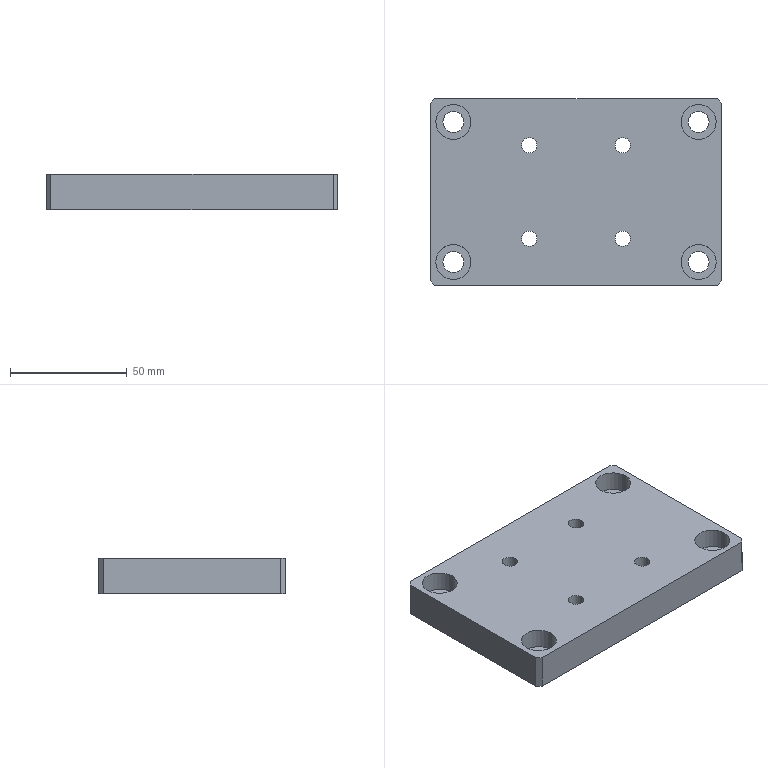Part | SolidWorks | features HoleWzd 2, Chamfer 1, Extrusion 1 | 1 solid | 50 faces | box 125 x 80 x 15 mm | volume 138563 mm3 | cylinder 32 | plane 18 | commonest cylinder face diameters 6.6 x8 9 x8 11 x8 15 x8
STEP:
#1=CARTESIAN_POINT('',(25.5,-20.,-1.1));
#2=VERTEX_POINT('',#1);
#3=CARTESIAN_POINT('',(14.5,-20.,-1.1));
#4=VERTEX_POINT('',#3);
#5=CARTESIAN_POINT('',(20.,-20.,-1.1));
#6=DIRECTION('',(0.,0.,-1.));
#7=DIRECTION('',(-1.,0.,0.));
#8=AXIS2_PLACEMENT_3D('',#5,#6,#7);
#9=CIRCLE('',#8,5.5);
#10=EDGE_CURVE('',#2,#4,#9,.T.);
#11=ORIENTED_EDGE('',*,*,#10,.F.);
#12=CARTESIAN_POINT('',(25.5,-20.,-7.5));
#13=VERTEX_POINT('',#12);
#14=CARTESIAN_POINT('',(25.5,-20.,-7.5));
#15=DIRECTION('',(0.,0.,-1.));
#16=VECTOR('',#15,1000.);
#17=LINE('',#14,#16);
#18=EDGE_CURVE('',#2,#13,#17,.T.);
#19=ORIENTED_EDGE('',*,*,#18,.T.);
#20=CARTESIAN_POINT('',(14.5,-20.,-7.5));
#21=VERTEX_POINT('',#20);
#22=CARTESIAN_POINT('',(20.,-20.,-7.5));
#23=DIRECTION('',(0.,0.,-1.));
#24=DIRECTION('',(-1.,0.,0.));
#25=AXIS2_PLACEMENT_3D('',#22,#23,#24);
#26=CIRCLE('',#25,5.5);
#27=EDGE_CURVE('',#13,#21,#26,.T.);
#28=ORIENTED_EDGE('',*,*,#27,.T.);
#29=CARTESIAN_POINT('',(14.5,-20.,-7.5));
#30=DIRECTION('',(0.,0.,-1.));
#31=VECTOR('',#30,1000.);
#32=LINE('',#29,#31);
#33=EDGE_CURVE('',#4,#21,#32,.T.);
#34=ORIENTED_EDGE('',*,*,#33,.F.);
#35=EDGE_LOOP('',(#11,#19,#28,#34));
#36=FACE_OUTER_BOUND('',#35,.T.);
#37=CARTESIAN_POINT('',(20.,-20.,-7.5));
#38=DIRECTION('',(0.,0.,-1.));
#39=DIRECTION('',(-1.,0.,0.));
#40=AXIS2_PLACEMENT_3D('',#37,#38,#39);
#41=CYLINDRICAL_SURFACE('',#40,5.5);
#42=ADVANCED_FACE('',(#36),#41,.F.);
#43=CARTESIAN_POINT('',(23.3,-20.,7.5));
#44=VERTEX_POINT('',#43);
#45=CARTESIAN_POINT('',(16.7,-20.,7.5));
#46=VERTEX_POINT('',#45);
#47=CARTESIAN_POINT('',(20.,-20.,7.5));
#48=DIRECTION('',(0.,0.,-1.));
#49=DIRECTION('',(-1.,0.,0.));
#50=AXIS2_PLACEMENT_3D('',#47,#48,#49);
#51=CIRCLE('',#50,3.3);
#52=EDGE_CURVE('',#44,#46,#51,.T.);
#53=ORIENTED_EDGE('',*,*,#52,.F.);
#54=CARTESIAN_POINT('',(23.3,-20.,-1.1));
#55=VERTEX_POINT('',#54);
#56=CARTESIAN_POINT('',(23.3,-20.,-7.5));
#57=DIRECTION('',(0.,0.,-1.));
#58=VECTOR('',#57,1000.);
#59=LINE('',#56,#58);
#60=EDGE_CURVE('',#44,#55,#59,.T.);
#61=ORIENTED_EDGE('',*,*,#60,.T.);
#62=CARTESIAN_POINT('',(16.7,-20.,-1.1));
#63=VERTEX_POINT('',#62);
#64=CARTESIAN_POINT('',(20.,-20.,-1.1));
#65=DIRECTION('',(0.,0.,-1.));
#66=DIRECTION('',(-1.,0.,0.));
#67=AXIS2_PLACEMENT_3D('',#64,#65,#66);
#68=CIRCLE('',#67,3.3);
#69=EDGE_CURVE('',#55,#63,#68,.T.);
#70=ORIENTED_EDGE('',*,*,#69,.T.);
#71=CARTESIAN_POINT('',(16.7,-20.,-7.5));
#72=DIRECTION('',(0.,0.,-1.));
#73=VECTOR('',#72,1000.);
#74=LINE('',#71,#73);
#75=EDGE_CURVE('',#46,#63,#74,.T.);
#76=ORIENTED_EDGE('',*,*,#75,.F.);
#77=EDGE_LOOP('',(#53,#61,#70,#76));
#78=FACE_OUTER_BOUND('',#77,.T.);
#79=CARTESIAN_POINT('',(20.,-20.,-7.5));
#80=DIRECTION('',(0.,0.,-1.));
#81=DIRECTION('',(-1.,0.,0.));
#82=AXIS2_PLACEMENT_3D('',#79,#80,#81);
#83=CYLINDRICAL_SURFACE('',#82,3.3);
#84=ADVANCED_FACE('',(#78),#83,.F.);
#85=CARTESIAN_POINT('',(25.5,20.,-1.1));
#86=VERTEX_POINT('',#85);
#87=CARTESIAN_POINT('',(14.5,20.,-1.1));
#88=VERTEX_POINT('',#87);
#89=CARTESIAN_POINT('',(20.,20.,-1.1));
#90=DIRECTION('',(0.,0.,-1.));
#91=DIRECTION('',(-1.,0.,0.));
#92=AXIS2_PLACEMENT_3D('',#89,#90,#91);
#93=CIRCLE('',#92,5.5);
#94=EDGE_CURVE('',#86,#88,#93,.T.);
#95=ORIENTED_EDGE('',*,*,#94,.F.);
#96=CARTESIAN_POINT('',(25.5,20.,-7.5));
#97=VERTEX_POINT('',#96);
#98=CARTESIAN_POINT('',(25.5,20.,-7.5));
#99=DIRECTION('',(0.,0.,-1.));
#100=VECTOR('',#99,1000.);
#101=LINE('',#98,#100);
#102=EDGE_CURVE('',#86,#97,#101,.T.);
#103=ORIENTED_EDGE('',*,*,#102,.T.);
#104=CARTESIAN_POINT('',(14.5,20.,-7.5));
#105=VERTEX_POINT('',#104);
#106=CARTESIAN_POINT('',(20.,20.,-7.5));
#107=DIRECTION('',(0.,0.,-1.));
#108=DIRECTION('',(-1.,0.,0.));
#109=AXIS2_PLACEMENT_3D('',#106,#107,#108);
#110=CIRCLE('',#109,5.5);
#111=EDGE_CURVE('',#97,#105,#110,.T.);
#112=ORIENTED_EDGE('',*,*,#111,.T.);
#113=CARTESIAN_POINT('',(14.5,20.,-7.5));
#114=DIRECTION('',(0.,0.,-1.));
#115=VECTOR('',#114,1000.);
#116=LINE('',#113,#115);
#117=EDGE_CURVE('',#88,#105,#116,.T.);
#118=ORIENTED_EDGE('',*,*,#117,.F.);
#119=EDGE_LOOP('',(#95,#103,#112,#118));
#120=FACE_OUTER_BOUND('',#119,.T.);
#121=CARTESIAN_POINT('',(20.,20.,-7.5));
#122=DIRECTION('',(0.,0.,-1.));
#123=DIRECTION('',(-1.,0.,0.));
#124=AXIS2_PLACEMENT_3D('',#121,#122,#123);
#125=CYLINDRICAL_SURFACE('',#124,5.5);
#126=ADVANCED_FACE('',(#120),#125,.F.);
#127=CARTESIAN_POINT('',(23.3,20.,7.5));
#128=VERTEX_POINT('',#127);
#129=CARTESIAN_POINT('',(16.7,20.,7.5));
#130=VERTEX_POINT('',#129);
#131=CARTESIAN_POINT('',(20.,20.,7.5));
#132=DIRECTION('',(0.,0.,-1.));
#133=DIRECTION('',(-1.,0.,0.));
#134=AXIS2_PLACEMENT_3D('',#131,#132,#133);
#135=CIRCLE('',#134,3.3);
#136=EDGE_CURVE('',#128,#130,#135,.T.);
#137=ORIENTED_EDGE('',*,*,#136,.F.);
#138=CARTESIAN_POINT('',(23.3,20.,-1.1));
#139=VERTEX_POINT('',#138);
#140=CARTESIAN_POINT('',(23.3,20.,-7.5));
#141=DIRECTION('',(0.,0.,-1.));
#142=VECTOR('',#141,1000.);
#143=LINE('',#140,#142);
#144=EDGE_CURVE('',#128,#139,#143,.T.);
#145=ORIENTED_EDGE('',*,*,#144,.T.);
#146=CARTESIAN_POINT('',(16.7,20.,-1.1));
#147=VERTEX_POINT('',#146);
#148=CARTESIAN_POINT('',(20.,20.,-1.1));
#149=DIRECTION('',(0.,0.,-1.));
#150=DIRECTION('',(-1.,0.,0.));
#151=AXIS2_PLACEMENT_3D('',#148,#149,#150);
#152=CIRCLE('',#151,3.3);
#153=EDGE_CURVE('',#139,#147,#152,.T.);
#154=ORIENTED_EDGE('',*,*,#153,.T.);
#155=CARTESIAN_POINT('',(16.7,20.,-7.5));
#156=DIRECTION('',(0.,0.,-1.));
#157=VECTOR('',#156,1000.);
#158=LINE('',#155,#157);
#159=EDGE_CURVE('',#130,#147,#158,.T.);
#160=ORIENTED_EDGE('',*,*,#159,.F.);
#161=EDGE_LOOP('',(#137,#145,#154,#160));
#162=FACE_OUTER_BOUND('',#161,.T.);
#163=CARTESIAN_POINT('',(20.,20.,-7.5));
#164=DIRECTION('',(0.,0.,-1.));
#165=DIRECTION('',(-1.,0.,0.));
#166=AXIS2_PLACEMENT_3D('',#163,#164,#165);
#167=CYLINDRICAL_SURFACE('',#166,3.3);
#168=ADVANCED_FACE('',(#162),#167,.F.);
#169=CARTESIAN_POINT('',(-14.5,-20.,-1.1));
#170=VERTEX_POINT('',#169);
#171=CARTESIAN_POINT('',(-25.5,-20.,-1.1));
#172=VERTEX_POINT('',#171);
#173=CARTESIAN_POINT('',(-20.,-20.,-1.1));
#174=DIRECTION('',(0.,0.,-1.));
#175=DIRECTION('',(-1.,0.,0.));
#176=AXIS2_PLACEMENT_3D('',#173,#174,#175);
#177=CIRCLE('',#176,5.5);
#178=EDGE_CURVE('',#170,#172,#177,.T.);
#179=ORIENTED_EDGE('',*,*,#178,.F.);
#180=CARTESIAN_POINT('',(-14.5,-20.,-7.5));
#181=VERTEX_POINT('',#180);
#182=CARTESIAN_POINT('',(-14.5,-20.,-7.5));
#183=DIRECTION('',(0.,0.,-1.));
#184=VECTOR('',#183,1000.);
#185=LINE('',#182,#184);
#186=EDGE_CURVE('',#170,#181,#185,.T.);
#187=ORIENTED_EDGE('',*,*,#186,.T.);
#188=CARTESIAN_POINT('',(-25.5,-20.,-7.5));
#189=VERTEX_POINT('',#188);
#190=CARTESIAN_POINT('',(-20.,-20.,-7.5));
#191=DIRECTION('',(0.,0.,-1.));
#192=DIRECTION('',(-1.,0.,0.));
#193=AXIS2_PLACEMENT_3D('',#190,#191,#192);
#194=CIRCLE('',#193,5.5);
#195=EDGE_CURVE('',#181,#189,#194,.T.);
#196=ORIENTED_EDGE('',*,*,#195,.T.);
#197=CARTESIAN_POINT('',(-25.5,-20.,-7.5));
#198=DIRECTION('',(0.,0.,-1.));
#199=VECTOR('',#198,1000.);
#200=LINE('',#197,#199);
#201=EDGE_CURVE('',#172,#189,#200,.T.);
#202=ORIENTED_EDGE('',*,*,#201,.F.);
#203=EDGE_LOOP('',(#179,#187,#196,#202));
#204=FACE_OUTER_BOUND('',#203,.T.);
#205=CARTESIAN_POINT('',(-20.,-20.,-7.5));
#206=DIRECTION('',(0.,0.,-1.));
#207=DIRECTION('',(-1.,0.,0.));
#208=AXIS2_PLACEMENT_3D('',#205,#206,#207);
#209=CYLINDRICAL_SURFACE('',#208,5.5);
#210=ADVANCED_FACE('',(#204),#209,.F.);
#211=CARTESIAN_POINT('',(-16.7,-20.,7.5));
#212=VERTEX_POINT('',#211);
#213=CARTESIAN_POINT('',(-23.3,-20.,7.5));
#214=VERTEX_POINT('',#213);
#215=CARTESIAN_POINT('',(-20.,-20.,7.5));
#216=DIRECTION('',(0.,0.,-1.));
#217=DIRECTION('',(-1.,0.,0.));
#218=AXIS2_PLACEMENT_3D('',#215,#216,#217);
#219=CIRCLE('',#218,3.3);
#220=EDGE_CURVE('',#212,#214,#219,.T.);
#221=ORIENTED_EDGE('',*,*,#220,.F.);
#222=CARTESIAN_POINT('',(-16.7,-20.,-1.1));
#223=VERTEX_POINT('',#222);
#224=CARTESIAN_POINT('',(-16.7,-20.,-7.5));
#225=DIRECTION('',(0.,0.,-1.));
#226=VECTOR('',#225,1000.);
#227=LINE('',#224,#226);
#228=EDGE_CURVE('',#212,#223,#227,.T.);
#229=ORIENTED_EDGE('',*,*,#228,.T.);
#230=CARTESIAN_POINT('',(-23.3,-20.,-1.1));
#231=VERTEX_POINT('',#230);
#232=CARTESIAN_POINT('',(-20.,-20.,-1.1));
#233=DIRECTION('',(0.,0.,-1.));
#234=DIRECTION('',(-1.,0.,0.));
#235=AXIS2_PLACEMENT_3D('',#232,#233,#234);
#236=CIRCLE('',#235,3.3);
#237=EDGE_CURVE('',#223,#231,#236,.T.);
#238=ORIENTED_EDGE('',*,*,#237,.T.);
#239=CARTESIAN_POINT('',(-23.3,-20.,-7.5));
#240=DIRECTION('',(0.,0.,-1.));
#241=VECTOR('',#240,1000.);
#242=LINE('',#239,#241);
#243=EDGE_CURVE('',#214,#231,#242,.T.);
#244=ORIENTED_EDGE('',*,*,#243,.F.);
#245=EDGE_LOOP('',(#221,#229,#238,#244));
#246=FACE_OUTER_BOUND('',#245,.T.);
#247=CARTESIAN_POINT('',(-20.,-20.,-7.5));
#248=DIRECTION('',(0.,0.,-1.));
#249=DIRECTION('',(-1.,0.,0.));
#250=AXIS2_PLACEMENT_3D('',#247,#248,#249);
#251=CYLINDRICAL_SURFACE('',#250,3.3);
#252=ADVANCED_FACE('',(#246),#251,.F.);
#253=CARTESIAN_POINT('',(-14.5,20.,-1.1));
#254=VERTEX_POINT('',#253);
#255=CARTESIAN_POINT('',(-25.5,20.,-1.1));
#256=VERTEX_POINT('',#255);
#257=CARTESIAN_POINT('',(-20.,20.,-1.1));
#258=DIRECTION('',(0.,0.,-1.));
#259=DIRECTION('',(-1.,0.,0.));
#260=AXIS2_PLACEMENT_3D('',#257,#258,#259);
#261=CIRCLE('',#260,5.5);
#262=EDGE_CURVE('',#254,#256,#261,.T.);
#263=ORIENTED_EDGE('',*,*,#262,.F.);
#264=CARTESIAN_POINT('',(-14.5,20.,-7.5));
#265=VERTEX_POINT('',#264);
#266=CARTESIAN_POINT('',(-14.5,20.,-7.5));
#267=DIRECTION('',(0.,0.,-1.));
#268=VECTOR('',#267,1000.);
#269=LINE('',#266,#268);
#270=EDGE_CURVE('',#254,#265,#269,.T.);
#271=ORIENTED_EDGE('',*,*,#270,.T.);
#272=CARTESIAN_POINT('',(-25.5,20.,-7.5));
#273=VERTEX_POINT('',#272);
#274=CARTESIAN_POINT('',(-20.,20.,-7.5));
#275=DIRECTION('',(0.,0.,-1.));
#276=DIRECTION('',(-1.,0.,0.));
#277=AXIS2_PLACEMENT_3D('',#274,#275,#276);
#278=CIRCLE('',#277,5.5);
#279=EDGE_CURVE('',#265,#273,#278,.T.);
#280=ORIENTED_EDGE('',*,*,#279,.T.);
#281=CARTESIAN_POINT('',(-25.5,20.,-7.5));
#282=DIRECTION('',(0.,0.,-1.));
#283=VECTOR('',#282,1000.);
#284=LINE('',#281,#283);
#285=EDGE_CURVE('',#256,#273,#284,.T.);
#286=ORIENTED_EDGE('',*,*,#285,.F.);
#287=EDGE_LOOP('',(#263,#271,#280,#286));
#288=FACE_OUTER_BOUND('',#287,.T.);
#289=CARTESIAN_POINT('',(-20.,20.,-7.5));
#290=DIRECTION('',(0.,0.,-1.));
#291=DIRECTION('',(-1.,0.,0.));
#292=AXIS2_PLACEMENT_3D('',#289,#290,#291);
#293=CYLINDRICAL_SURFACE('',#292,5.5);
#294=ADVANCED_FACE('',(#288),#293,.F.);
#295=CARTESIAN_POINT('',(-16.7,20.,7.5));
#296=VERTEX_POINT('',#295);
#297=CARTESIAN_POINT('',(-23.3,20.,7.5));
#298=VERTEX_POINT('',#297);
#299=CARTESIAN_POINT('',(-20.,20.,7.5));
#300=DIRECTION('',(0.,0.,-1.));
#301=DIRECTION('',(-1.,0.,0.));
#302=AXIS2_PLACEMENT_3D('',#299,#300,#301);
#303=CIRCLE('',#302,3.3);
#304=EDGE_CURVE('',#296,#298,#303,.T.);
#305=ORIENTED_EDGE('',*,*,#304,.F.);
#306=CARTESIAN_POINT('',(-16.7,20.,-1.1));
#307=VERTEX_POINT('',#306);
#308=CARTESIAN_POINT('',(-16.7,20.,-7.5));
#309=DIRECTION('',(0.,0.,-1.));
#310=VECTOR('',#309,1000.);
#311=LINE('',#308,#310);
#312=EDGE_CURVE('',#296,#307,#311,.T.);
#313=ORIENTED_EDGE('',*,*,#312,.T.);
#314=CARTESIAN_POINT('',(-23.3,20.,-1.1));
#315=VERTEX_POINT('',#314);
#316=CARTESIAN_POINT('',(-20.,20.,-1.1));
#317=DIRECTION('',(0.,0.,-1.));
#318=DIRECTION('',(-1.,0.,0.));
#319=AXIS2_PLACEMENT_3D('',#316,#317,#318);
#320=CIRCLE('',#319,3.3);
#321=EDGE_CURVE('',#307,#315,#320,.T.);
#322=ORIENTED_EDGE('',*,*,#321,.T.);
#323=CARTESIAN_POINT('',(-23.3,20.,-7.5));
#324=DIRECTION('',(0.,0.,-1.));
#325=VECTOR('',#324,1000.);
#326=LINE('',#323,#325);
#327=EDGE_CURVE('',#298,#315,#326,.T.);
#328=ORIENTED_EDGE('',*,*,#327,.F.);
#329=EDGE_LOOP('',(#305,#313,#322,#328));
#330=FACE_OUTER_BOUND('',#329,.T.);
#331=CARTESIAN_POINT('',(-20.,20.,-7.5));
#332=DIRECTION('',(0.,0.,-1.));
#333=DIRECTION('',(-1.,0.,0.));
#334=AXIS2_PLACEMENT_3D('',#331,#332,#333);
#335=CYLINDRICAL_SURFACE('',#334,3.3);
#336=ADVANCED_FACE('',(#330),#335,.F.);
#337=CARTESIAN_POINT('',(-60.,30.,-1.1));
#338=VERTEX_POINT('',#337);
#339=CARTESIAN_POINT('',(-45.,30.,-1.1));
#340=VERTEX_POINT('',#339);
#341=CARTESIAN_POINT('',(-52.5,30.,-1.1));
#342=DIRECTION('',(0.,0.,1.));
#343=DIRECTION('',(1.,0.,0.));
#344=AXIS2_PLACEMENT_3D('',#341,#342,#343);
#345=CIRCLE('',#344,7.5);
#346=EDGE_CURVE('',#338,#340,#345,.T.);
#347=ORIENTED_EDGE('',*,*,#346,.F.);
#348=CARTESIAN_POINT('',(-60.,30.,7.5));
#349=VERTEX_POINT('',#348);
#350=CARTESIAN_POINT('',(-60.,30.,7.5));
#351=DIRECTION('',(0.,0.,1.));
#352=VECTOR('',#351,1000.);
#353=LINE('',#350,#352);
#354=EDGE_CURVE('',#338,#349,#353,.T.);
#355=ORIENTED_EDGE('',*,*,#354,.T.);
#356=CARTESIAN_POINT('',(-45.,30.,7.5));
#357=VERTEX_POINT('',#356);
#358=CARTESIAN_POINT('',(-52.5,30.,7.5));
#359=DIRECTION('',(0.,0.,1.));
#360=DIRECTION('',(1.,0.,0.));
#361=AXIS2_PLACEMENT_3D('',#358,#359,#360);
#362=CIRCLE('',#361,7.5);
#363=EDGE_CURVE('',#349,#357,#362,.T.);
#364=ORIENTED_EDGE('',*,*,#363,.T.);
#365=CARTESIAN_POINT('',(-45.,30.,7.5));
#366=DIRECTION('',(0.,0.,1.));
#367=VECTOR('',#366,1000.);
#368=LINE('',#365,#367);
#369=EDGE_CURVE('',#340,#357,#368,.T.);
#370=ORIENTED_EDGE('',*,*,#369,.F.);
#371=EDGE_LOOP('',(#347,#355,#364,#370));
#372=FACE_OUTER_BOUND('',#371,.T.);
#373=CARTESIAN_POINT('',(-52.5,30.,7.5));
#374=DIRECTION('',(0.,0.,1.));
#375=DIRECTION('',(1.,0.,0.));
#376=AXIS2_PLACEMENT_3D('',#373,#374,#375);
#377=CYLINDRICAL_SURFACE('',#376,7.5);
#378=ADVANCED_FACE('',(#372),#377,.F.);
#379=CARTESIAN_POINT('',(-57.,30.,-7.5));
#380=VERTEX_POINT('',#379);
#381=CARTESIAN_POINT('',(-48.,30.,-7.5));
#382=VERTEX_POINT('',#381);
#383=CARTESIAN_POINT('',(-52.5,30.,-7.5));
#384=DIRECTION('',(0.,0.,1.));
#385=DIRECTION('',(1.,0.,0.));
#386=AXIS2_PLACEMENT_3D('',#383,#384,#385);
#387=CIRCLE('',#386,4.5);
#388=EDGE_CURVE('',#380,#382,#387,.T.);
#389=ORIENTED_EDGE('',*,*,#388,.F.);
#390=CARTESIAN_POINT('',(-57.,30.,-1.1));
#391=VERTEX_POINT('',#390);
#392=CARTESIAN_POINT('',(-57.,30.,7.5));
#393=DIRECTION('',(0.,0.,1.));
#394=VECTOR('',#393,1000.);
#395=LINE('',#392,#394);
#396=EDGE_CURVE('',#380,#391,#395,.T.);
#397=ORIENTED_EDGE('',*,*,#396,.T.);
#398=CARTESIAN_POINT('',(-48.,30.,-1.1));
#399=VERTEX_POINT('',#398);
#400=CARTESIAN_POINT('',(-52.5,30.,-1.1));
#401=DIRECTION('',(0.,0.,1.));
#402=DIRECTION('',(1.,0.,0.));
#403=AXIS2_PLACEMENT_3D('',#400,#401,#402);
#404=CIRCLE('',#403,4.5);
#405=EDGE_CURVE('',#391,#399,#404,.T.);
#406=ORIENTED_EDGE('',*,*,#405,.T.);
#407=CARTESIAN_POINT('',(-48.,30.,7.5));
#408=DIRECTION('',(0.,0.,1.));
#409=VECTOR('',#408,1000.);
#410=LINE('',#407,#409);
#411=EDGE_CURVE('',#382,#399,#410,.T.);
#412=ORIENTED_EDGE('',*,*,#411,.F.);
#413=EDGE_LOOP('',(#389,#397,#406,#412));
#414=FACE_OUTER_BOUND('',#413,.T.);
#415=CARTESIAN_POINT('',(-52.5,30.,7.5));
#416=DIRECTION('',(0.,0.,1.));
#417=DIRECTION('',(1.,0.,0.));
#418=AXIS2_PLACEMENT_3D('',#415,#416,#417);
#419=CYLINDRICAL_SURFACE('',#418,4.5);
#420=ADVANCED_FACE('',(#414),#419,.F.);
#421=CARTESIAN_POINT('',(-60.,-30.,-1.1));
#422=VERTEX_POINT('',#421);
#423=CARTESIAN_POINT('',(-45.,-30.,-1.1));
#424=VERTEX_POINT('',#423);
#425=CARTESIAN_POINT('',(-52.5,-30.,-1.1));
#426=DIRECTION('',(0.,0.,1.));
#427=DIRECTION('',(1.,0.,0.));
#428=AXIS2_PLACEMENT_3D('',#425,#426,#427);
#429=CIRCLE('',#428,7.5);
#430=EDGE_CURVE('',#422,#424,#429,.T.);
#431=ORIENTED_EDGE('',*,*,#430,.F.);
#432=CARTESIAN_POINT('',(-60.,-30.,7.5));
#433=VERTEX_POINT('',#432);
#434=CARTESIAN_POINT('',(-60.,-30.,7.5));
#435=DIRECTION('',(0.,0.,1.));
#436=VECTOR('',#435,1000.);
#437=LINE('',#434,#436);
#438=EDGE_CURVE('',#422,#433,#437,.T.);
#439=ORIENTED_EDGE('',*,*,#438,.T.);
#440=CARTESIAN_POINT('',(-45.,-30.,7.5));
#441=VERTEX_POINT('',#440);
#442=CARTESIAN_POINT('',(-52.5,-30.,7.5));
#443=DIRECTION('',(0.,0.,1.));
#444=DIRECTION('',(1.,0.,0.));
#445=AXIS2_PLACEMENT_3D('',#442,#443,#444);
#446=CIRCLE('',#445,7.5);
#447=EDGE_CURVE('',#433,#441,#446,.T.);
#448=ORIENTED_EDGE('',*,*,#447,.T.);
#449=CARTESIAN_POINT('',(-45.,-30.,7.5));
#450=DIRECTION('',(0.,0.,1.));
#451=VECTOR('',#450,1000.);
#452=LINE('',#449,#451);
#453=EDGE_CURVE('',#424,#441,#452,.T.);
#454=ORIENTED_EDGE('',*,*,#453,.F.);
#455=EDGE_LOOP('',(#431,#439,#448,#454));
#456=FACE_OUTER_BOUND('',#455,.T.);
#457=CARTESIAN_POINT('',(-52.5,-30.,7.5));
#458=DIRECTION('',(0.,0.,1.));
#459=DIRECTION('',(1.,0.,0.));
#460=AXIS2_PLACEMENT_3D('',#457,#458,#459);
#461=CYLINDRICAL_SURFACE('',#460,7.5);
#462=ADVANCED_FACE('',(#456),#461,.F.);
#463=CARTESIAN_POINT('',(-57.,-30.,-7.5));
#464=VERTEX_POINT('',#463);
#465=CARTESIAN_POINT('',(-48.,-30.,-7.5));
#466=VERTEX_POINT('',#465);
#467=CARTESIAN_POINT('',(-52.5,-30.,-7.5));
#468=DIRECTION('',(0.,0.,1.));
#469=DIRECTION('',(1.,0.,0.));
#470=AXIS2_PLACEMENT_3D('',#467,#468,#469);
#471=CIRCLE('',#470,4.5);
#472=EDGE_CURVE('',#464,#466,#471,.T.);
#473=ORIENTED_EDGE('',*,*,#472,.F.);
#474=CARTESIAN_POINT('',(-57.,-30.,-1.1));
#475=VERTEX_POINT('',#474);
#476=CARTESIAN_POINT('',(-57.,-30.,7.5));
#477=DIRECTION('',(0.,0.,1.));
#478=VECTOR('',#477,1000.);
#479=LINE('',#476,#478);
#480=EDGE_CURVE('',#464,#475,#479,.T.);
#481=ORIENTED_EDGE('',*,*,#480,.T.);
#482=CARTESIAN_POINT('',(-48.,-30.,-1.1));
#483=VERTEX_POINT('',#482);
#484=CARTESIAN_POINT('',(-52.5,-30.,-1.1));
#485=DIRECTION('',(0.,0.,1.));
#486=DIRECTION('',(1.,0.,0.));
#487=AXIS2_PLACEMENT_3D('',#484,#485,#486);
#488=CIRCLE('',#487,4.5);
#489=EDGE_CURVE('',#475,#483,#488,.T.);
#490=ORIENTED_EDGE('',*,*,#489,.T.);
#491=CARTESIAN_POINT('',(-48.,-30.,7.5));
#492=DIRECTION('',(0.,0.,1.));
#493=VECTOR('',#492,1000.);
#494=LINE('',#491,#493);
#495=EDGE_CURVE('',#466,#483,#494,.T.);
#496=ORIENTED_EDGE('',*,*,#495,.F.);
#497=EDGE_LOOP('',(#473,#481,#490,#496));
#498=FACE_OUTER_BOUND('',#497,.T.);
#499=CARTESIAN_POINT('',(-52.5,-30.,7.5));
#500=DIRECTION('',(0.,0.,1.));
#501=DIRECTION('',(1.,0.,0.));
#502=AXIS2_PLACEMENT_3D('',#499,#500,#501);
#503=CYLINDRICAL_SURFACE('',#502,4.5);
#504=ADVANCED_FACE('',(#498),#503,.F.);
#505=CARTESIAN_POINT('',(45.,-30.,-1.1));
#506=VERTEX_POINT('',#505);
#507=CARTESIAN_POINT('',(60.,-30.,-1.1));
#508=VERTEX_POINT('',#507);
#509=CARTESIAN_POINT('',(52.5,-30.,-1.1));
#510=DIRECTION('',(0.,0.,1.));
#511=DIRECTION('',(1.,0.,0.));
#512=AXIS2_PLACEMENT_3D('',#509,#510,#511);
#513=CIRCLE('',#512,7.5);
#514=EDGE_CURVE('',#506,#508,#513,.T.);
#515=ORIENTED_EDGE('',*,*,#514,.F.);
#516=CARTESIAN_POINT('',(45.,-30.,7.5));
#517=VERTEX_POINT('',#516);
#518=CARTESIAN_POINT('',(45.,-30.,7.5));
#519=DIRECTION('',(0.,0.,1.));
#520=VECTOR('',#519,1000.);
#521=LINE('',#518,#520);
#522=EDGE_CURVE('',#506,#517,#521,.T.);
#523=ORIENTED_EDGE('',*,*,#522,.T.);
#524=CARTESIAN_POINT('',(60.,-30.,7.5));
#525=VERTEX_POINT('',#524);
#526=CARTESIAN_POINT('',(52.5,-30.,7.5));
#527=DIRECTION('',(0.,0.,1.));
#528=DIRECTION('',(1.,0.,0.));
#529=AXIS2_PLACEMENT_3D('',#526,#527,#528);
#530=CIRCLE('',#529,7.5);
#531=EDGE_CURVE('',#517,#525,#530,.T.);
#532=ORIENTED_EDGE('',*,*,#531,.T.);
#533=CARTESIAN_POINT('',(60.,-30.,7.5));
#534=DIRECTION('',(0.,0.,1.));
#535=VECTOR('',#534,1000.);
#536=LINE('',#533,#535);
#537=EDGE_CURVE('',#508,#525,#536,.T.);
#538=ORIENTED_EDGE('',*,*,#537,.F.);
#539=EDGE_LOOP('',(#515,#523,#532,#538));
#540=FACE_OUTER_BOUND('',#539,.T.);
#541=CARTESIAN_POINT('',(52.5,-30.,7.5));
#542=DIRECTION('',(0.,0.,1.));
#543=DIRECTION('',(1.,0.,0.));
#544=AXIS2_PLACEMENT_3D('',#541,#542,#543);
#545=CYLINDRICAL_SURFACE('',#544,7.5);
#546=ADVANCED_FACE('',(#540),#545,.F.);
#547=CARTESIAN_POINT('',(48.,-30.,-7.5));
#548=VERTEX_POINT('',#547);
#549=CARTESIAN_POINT('',(57.,-30.,-7.5));
#550=VERTEX_POINT('',#549);
#551=CARTESIAN_POINT('',(52.5,-30.,-7.5));
#552=DIRECTION('',(0.,0.,1.));
#553=DIRECTION('',(1.,0.,0.));
#554=AXIS2_PLACEMENT_3D('',#551,#552,#553);
#555=CIRCLE('',#554,4.5);
#556=EDGE_CURVE('',#548,#550,#555,.T.);
#557=ORIENTED_EDGE('',*,*,#556,.F.);
#558=CARTESIAN_POINT('',(48.,-30.,-1.1));
#559=VERTEX_POINT('',#558);
#560=CARTESIAN_POINT('',(48.,-30.,7.5));
#561=DIRECTION('',(0.,0.,1.));
#562=VECTOR('',#561,1000.);
#563=LINE('',#560,#562);
#564=EDGE_CURVE('',#548,#559,#563,.T.);
#565=ORIENTED_EDGE('',*,*,#564,.T.);
#566=CARTESIAN_POINT('',(57.,-30.,-1.1));
#567=VERTEX_POINT('',#566);
#568=CARTESIAN_POINT('',(52.5,-30.,-1.1));
#569=DIRECTION('',(0.,0.,1.));
#570=DIRECTION('',(1.,0.,0.));
#571=AXIS2_PLACEMENT_3D('',#568,#569,#570);
#572=CIRCLE('',#571,4.5);
#573=EDGE_CURVE('',#559,#567,#572,.T.);
#574=ORIENTED_EDGE('',*,*,#573,.T.);
#575=CARTESIAN_POINT('',(57.,-30.,7.5));
#576=DIRECTION('',(0.,0.,1.));
#577=VECTOR('',#576,1000.);
#578=LINE('',#575,#577);
#579=EDGE_CURVE('',#550,#567,#578,.T.);
#580=ORIENTED_EDGE('',*,*,#579,.F.);
#581=EDGE_LOOP('',(#557,#565,#574,#580));
#582=FACE_OUTER_BOUND('',#581,.T.);
#583=CARTESIAN_POINT('',(52.5,-30.,7.5));
#584=DIRECTION('',(0.,0.,1.));
#585=DIRECTION('',(1.,0.,0.));
#586=AXIS2_PLACEMENT_3D('',#583,#584,#585);
#587=CYLINDRICAL_SURFACE('',#586,4.5);
#588=ADVANCED_FACE('',(#582),#587,.F.);
#589=CARTESIAN_POINT('',(45.,30.,-1.1));
#590=VERTEX_POINT('',#589);
#591=CARTESIAN_POINT('',(60.,30.,-1.1));
#592=VERTEX_POINT('',#591);
#593=CARTESIAN_POINT('',(52.5,30.,-1.1));
#594=DIRECTION('',(0.,0.,1.));
#595=DIRECTION('',(1.,0.,0.));
#596=AXIS2_PLACEMENT_3D('',#593,#594,#595);
#597=CIRCLE('',#596,7.5);
#598=EDGE_CURVE('',#590,#592,#597,.T.);
#599=ORIENTED_EDGE('',*,*,#598,.F.);
#600=CARTESIAN_POINT('',(45.,30.,7.5));
#601=VERTEX_POINT('',#600);
#602=CARTESIAN_POINT('',(45.,30.,7.5));
#603=DIRECTION('',(0.,0.,1.));
#604=VECTOR('',#603,1000.);
#605=LINE('',#602,#604);
#606=EDGE_CURVE('',#590,#601,#605,.T.);
#607=ORIENTED_EDGE('',*,*,#606,.T.);
#608=CARTESIAN_POINT('',(60.,30.,7.5));
#609=VERTEX_POINT('',#608);
#610=CARTESIAN_POINT('',(52.5,30.,7.5));
#611=DIRECTION('',(0.,0.,1.));
#612=DIRECTION('',(1.,0.,0.));
#613=AXIS2_PLACEMENT_3D('',#610,#611,#612);
#614=CIRCLE('',#613,7.5);
#615=EDGE_CURVE('',#601,#609,#614,.T.);
#616=ORIENTED_EDGE('',*,*,#615,.T.);
#617=CARTESIAN_POINT('',(60.,30.,7.5));
#618=DIRECTION('',(0.,0.,1.));
#619=VECTOR('',#618,1000.);
#620=LINE('',#617,#619);
#621=EDGE_CURVE('',#592,#609,#620,.T.);
#622=ORIENTED_EDGE('',*,*,#621,.F.);
#623=EDGE_LOOP('',(#599,#607,#616,#622));
#624=FACE_OUTER_BOUND('',#623,.T.);
#625=CARTESIAN_POINT('',(52.5,30.,7.5));
#626=DIRECTION('',(0.,0.,1.));
#627=DIRECTION('',(1.,0.,0.));
#628=AXIS2_PLACEMENT_3D('',#625,#626,#627);
#629=CYLINDRICAL_SURFACE('',#628,7.5);
#630=ADVANCED_FACE('',(#624),#629,.F.);
#631=CARTESIAN_POINT('',(48.,30.,-7.5));
#632=VERTEX_POINT('',#631);
#633=CARTESIAN_POINT('',(57.,30.,-7.5));
#634=VERTEX_POINT('',#633);
#635=CARTESIAN_POINT('',(52.5,30.,-7.5));
#636=DIRECTION('',(0.,0.,1.));
#637=DIRECTION('',(1.,0.,0.));
#638=AXIS2_PLACEMENT_3D('',#635,#636,#637);
#639=CIRCLE('',#638,4.5);
#640=EDGE_CURVE('',#632,#634,#639,.T.);
#641=ORIENTED_EDGE('',*,*,#640,.F.);
#642=CARTESIAN_POINT('',(48.,30.,-1.1));
#643=VERTEX_POINT('',#642);
#644=CARTESIAN_POINT('',(48.,30.,7.5));
#645=DIRECTION('',(0.,0.,1.));
#646=VECTOR('',#645,1000.);
#647=LINE('',#644,#646);
#648=EDGE_CURVE('',#632,#643,#647,.T.);
#649=ORIENTED_EDGE('',*,*,#648,.T.);
#650=CARTESIAN_POINT('',(57.,30.,-1.1));
#651=VERTEX_POINT('',#650);
#652=CARTESIAN_POINT('',(52.5,30.,-1.1));
#653=DIRECTION('',(0.,0.,1.));
#654=DIRECTION('',(1.,0.,0.));
#655=AXIS2_PLACEMENT_3D('',#652,#653,#654);
#656=CIRCLE('',#655,4.5);
#657=EDGE_CURVE('',#643,#651,#656,.T.);
#658=ORIENTED_EDGE('',*,*,#657,.T.);
#659=CARTESIAN_POINT('',(57.,30.,7.5));
#660=DIRECTION('',(0.,0.,1.));
#661=VECTOR('',#660,1000.);
#662=LINE('',#659,#661);
#663=EDGE_CURVE('',#634,#651,#662,.T.);
#664=ORIENTED_EDGE('',*,*,#663,.F.);
#665=EDGE_LOOP('',(#641,#649,#658,#664));
#666=FACE_OUTER_BOUND('',#665,.T.);
#667=CARTESIAN_POINT('',(52.5,30.,7.5));
#668=DIRECTION('',(0.,0.,1.));
#669=DIRECTION('',(1.,0.,0.));
#670=AXIS2_PLACEMENT_3D('',#667,#668,#669);
#671=CYLINDRICAL_SURFACE('',#670,4.5);
#672=ADVANCED_FACE('',(#666),#671,.F.);
#673=CARTESIAN_POINT('',(62.5,-38.,-7.5));
#674=VERTEX_POINT('',#673);
#675=CARTESIAN_POINT('',(62.5,38.,-7.5));
#676=VERTEX_POINT('',#675);
#677=CARTESIAN_POINT('',(62.5,40.,-7.5));
#678=DIRECTION('',(0.,1.,0.));
#679=VECTOR('',#678,1000.);
#680=LINE('',#677,#679);
#681=EDGE_CURVE('',#674,#676,#680,.T.);
#682=ORIENTED_EDGE('',*,*,#681,.T.);
#683=CARTESIAN_POINT('',(62.5,38.,7.5));
#684=VERTEX_POINT('',#683);
#685=CARTESIAN_POINT('',(62.5,38.,7.5));
#686=DIRECTION('',(0.,0.,1.));
#687=VECTOR('',#686,1000.);
#688=LINE('',#685,#687);
#689=EDGE_CURVE('',#676,#684,#688,.T.);
#690=ORIENTED_EDGE('',*,*,#689,.T.);
#691=CARTESIAN_POINT('',(62.5,-38.,7.5));
#692=VERTEX_POINT('',#691);
#693=CARTESIAN_POINT('',(62.5,40.,7.5));
#694=DIRECTION('',(0.,1.,0.));
#695=VECTOR('',#694,1000.);
#696=LINE('',#693,#695);
#697=EDGE_CURVE('',#692,#684,#696,.T.);
#698=ORIENTED_EDGE('',*,*,#697,.F.);
#699=CARTESIAN_POINT('',(62.5,-38.,7.5));
#700=DIRECTION('',(0.,0.,-1.));
#701=VECTOR('',#700,1000.);
#702=LINE('',#699,#701);
#703=EDGE_CURVE('',#692,#674,#702,.T.);
#704=ORIENTED_EDGE('',*,*,#703,.T.);
#705=EDGE_LOOP('',(#682,#690,#698,#704));
#706=FACE_OUTER_BOUND('',#705,.T.);
#707=CARTESIAN_POINT('',(62.5,40.,7.5));
#708=DIRECTION('',(-1.,0.,0.));
#709=DIRECTION('',(0.,-1.,0.));
#710=AXIS2_PLACEMENT_3D('',#707,#708,#709);
#711=PLANE('',#710);
#712=ADVANCED_FACE('',(#706),#711,.F.);
#713=CARTESIAN_POINT('',(60.5,40.,7.5));
#714=VERTEX_POINT('',#713);
#715=CARTESIAN_POINT('',(-60.5,40.,7.5));
#716=VERTEX_POINT('',#715);
#717=CARTESIAN_POINT('',(-62.5,40.,7.5));
#718=DIRECTION('',(-1.,0.,0.));
#719=VECTOR('',#718,1000.);
#720=LINE('',#717,#719);
#721=EDGE_CURVE('',#714,#716,#720,.T.);
#722=ORIENTED_EDGE('',*,*,#721,.F.);
#723=CARTESIAN_POINT('',(60.5,40.,-7.5));
#724=VERTEX_POINT('',#723);
#725=CARTESIAN_POINT('',(60.5,40.,7.5));
#726=DIRECTION('',(0.,0.,-1.));
#727=VECTOR('',#726,1000.);
#728=LINE('',#725,#727);
#729=EDGE_CURVE('',#714,#724,#728,.T.);
#730=ORIENTED_EDGE('',*,*,#729,.T.);
#731=CARTESIAN_POINT('',(-60.5,40.,-7.5));
#732=VERTEX_POINT('',#731);
#733=CARTESIAN_POINT('',(-62.5,40.,-7.5));
#734=DIRECTION('',(-1.,0.,0.));
#735=VECTOR('',#734,1000.);
#736=LINE('',#733,#735);
#737=EDGE_CURVE('',#724,#732,#736,.T.);
#738=ORIENTED_EDGE('',*,*,#737,.T.);
#739=CARTESIAN_POINT('',(-60.5,40.,7.5));
#740=DIRECTION('',(0.,0.,1.));
#741=VECTOR('',#740,1000.);
#742=LINE('',#739,#741);
#743=EDGE_CURVE('',#732,#716,#742,.T.);
#744=ORIENTED_EDGE('',*,*,#743,.T.);
#745=EDGE_LOOP('',(#722,#730,#738,#744));
#746=FACE_OUTER_BOUND('',#745,.T.);
#747=CARTESIAN_POINT('',(-62.5,40.,7.5));
#748=DIRECTION('',(0.,-1.,0.));
#749=DIRECTION('',(0.,0.,-1.));
#750=AXIS2_PLACEMENT_3D('',#747,#748,#749);
#751=PLANE('',#750);
#752=ADVANCED_FACE('',(#746),#751,.F.);
#753=CARTESIAN_POINT('',(-62.5,38.,-7.5));
#754=VERTEX_POINT('',#753);
#755=CARTESIAN_POINT('',(-62.5,-38.,-7.5));
#756=VERTEX_POINT('',#755);
#757=CARTESIAN_POINT('',(-62.5,40.,-7.5));
#758=DIRECTION('',(0.,-1.,0.));
#759=VECTOR('',#758,1000.);
#760=LINE('',#757,#759);
#761=EDGE_CURVE('',#754,#756,#760,.T.);
#762=ORIENTED_EDGE('',*,*,#761,.T.);
#763=CARTESIAN_POINT('',(-62.5,-38.,7.5));
#764=VERTEX_POINT('',#763);
#765=CARTESIAN_POINT('',(-62.5,-38.,7.5));
#766=DIRECTION('',(0.,0.,1.));
#767=VECTOR('',#766,1000.);
#768=LINE('',#765,#767);
#769=EDGE_CURVE('',#756,#764,#768,.T.);
#770=ORIENTED_EDGE('',*,*,#769,.T.);
#771=CARTESIAN_POINT('',(-62.5,38.,7.5));
#772=VERTEX_POINT('',#771);
#773=CARTESIAN_POINT('',(-62.5,40.,7.5));
#774=DIRECTION('',(0.,-1.,0.));
#775=VECTOR('',#774,1000.);
#776=LINE('',#773,#775);
#777=EDGE_CURVE('',#772,#764,#776,.T.);
#778=ORIENTED_EDGE('',*,*,#777,.F.);
#779=CARTESIAN_POINT('',(-62.5,38.,7.5));
#780=DIRECTION('',(0.,0.,-1.));
#781=VECTOR('',#780,1000.);
#782=LINE('',#779,#781);
#783=EDGE_CURVE('',#772,#754,#782,.T.);
#784=ORIENTED_EDGE('',*,*,#783,.T.);
#785=EDGE_LOOP('',(#762,#770,#778,#784));
#786=FACE_OUTER_BOUND('',#785,.T.);
#787=CARTESIAN_POINT('',(-62.5,40.,7.5));
#788=DIRECTION('',(1.,0.,0.));
#789=DIRECTION('',(0.,1.,0.));
#790=AXIS2_PLACEMENT_3D('',#787,#788,#789);
#791=PLANE('',#790);
#792=ADVANCED_FACE('',(#786),#791,.F.);
#793=CARTESIAN_POINT('',(-60.5,-40.,-7.5));
#794=VERTEX_POINT('',#793);
#795=CARTESIAN_POINT('',(60.5,-40.,-7.5));
#796=VERTEX_POINT('',#795);
#797=CARTESIAN_POINT('',(-62.5,-40.,-7.5));
#798=DIRECTION('',(1.,0.,0.));
#799=VECTOR('',#798,1000.);
#800=LINE('',#797,#799);
#801=EDGE_CURVE('',#794,#796,#800,.T.);
#802=ORIENTED_EDGE('',*,*,#801,.T.);
#803=CARTESIAN_POINT('',(60.5,-40.,7.5));
#804=VERTEX_POINT('',#803);
#805=CARTESIAN_POINT('',(60.5,-40.,7.5));
#806=DIRECTION('',(0.,0.,1.));
#807=VECTOR('',#806,1000.);
#808=LINE('',#805,#807);
#809=EDGE_CURVE('',#796,#804,#808,.T.);
#810=ORIENTED_EDGE('',*,*,#809,.T.);
#811=CARTESIAN_POINT('',(-60.5,-40.,7.5));
#812=VERTEX_POINT('',#811);
#813=CARTESIAN_POINT('',(-62.5,-40.,7.5));
#814=DIRECTION('',(1.,0.,0.));
#815=VECTOR('',#814,1000.);
#816=LINE('',#813,#815);
#817=EDGE_CURVE('',#812,#804,#816,.T.);
#818=ORIENTED_EDGE('',*,*,#817,.F.);
#819=CARTESIAN_POINT('',(-60.5,-40.,7.5));
#820=DIRECTION('',(0.,0.,-1.));
#821=VECTOR('',#820,1000.);
#822=LINE('',#819,#821);
#823=EDGE_CURVE('',#812,#794,#822,.T.);
#824=ORIENTED_EDGE('',*,*,#823,.T.);
#825=EDGE_LOOP('',(#802,#810,#818,#824));
#826=FACE_OUTER_BOUND('',#825,.T.);
#827=CARTESIAN_POINT('',(-62.5,-40.,7.5));
#828=DIRECTION('',(0.,1.,0.));
#829=DIRECTION('',(0.,0.,1.));
#830=AXIS2_PLACEMENT_3D('',#827,#828,#829);
#831=PLANE('',#830);
#832=ADVANCED_FACE('',(#826),#831,.F.);
#833=CARTESIAN_POINT('',(20.,-20.,7.5));
#834=DIRECTION('',(0.,0.,-1.));
#835=DIRECTION('',(-1.,0.,0.));
#836=AXIS2_PLACEMENT_3D('',#833,#834,#835);
#837=CIRCLE('',#836,3.3);
#838=EDGE_CURVE('',#46,#44,#837,.T.);
#839=ORIENTED_EDGE('',*,*,#838,.T.);
#840=ORIENTED_EDGE('',*,*,#52,.T.);
#841=EDGE_LOOP('',(#839,#840));
#842=FACE_BOUND('',#841,.T.);
#843=CARTESIAN_POINT('',(20.,20.,7.5));
#844=DIRECTION('',(0.,0.,-1.));
#845=DIRECTION('',(-1.,0.,0.));
#846=AXIS2_PLACEMENT_3D('',#843,#844,#845);
#847=CIRCLE('',#846,3.3);
#848=EDGE_CURVE('',#130,#128,#847,.T.);
#849=ORIENTED_EDGE('',*,*,#848,.T.);
#850=ORIENTED_EDGE('',*,*,#136,.T.);
#851=EDGE_LOOP('',(#849,#850));
#852=FACE_BOUND('',#851,.T.);
#853=CARTESIAN_POINT('',(-20.,-20.,7.5));
#854=DIRECTION('',(0.,0.,-1.));
#855=DIRECTION('',(-1.,0.,0.));
#856=AXIS2_PLACEMENT_3D('',#853,#854,#855);
#857=CIRCLE('',#856,3.3);
#858=EDGE_CURVE('',#214,#212,#857,.T.);
#859=ORIENTED_EDGE('',*,*,#858,.T.);
#860=ORIENTED_EDGE('',*,*,#220,.T.);
#861=EDGE_LOOP('',(#859,#860));
#862=FACE_BOUND('',#861,.T.);
#863=CARTESIAN_POINT('',(-20.,20.,7.5));
#864=DIRECTION('',(0.,0.,-1.));
#865=DIRECTION('',(-1.,0.,0.));
#866=AXIS2_PLACEMENT_3D('',#863,#864,#865);
#867=CIRCLE('',#866,3.3);
#868=EDGE_CURVE('',#298,#296,#867,.T.);
#869=ORIENTED_EDGE('',*,*,#868,.T.);
#870=ORIENTED_EDGE('',*,*,#304,.T.);
#871=EDGE_LOOP('',(#869,#870));
#872=FACE_BOUND('',#871,.T.);
#873=CARTESIAN_POINT('',(-52.5,30.,7.5));
#874=DIRECTION('',(0.,0.,1.));
#875=DIRECTION('',(1.,0.,0.));
#876=AXIS2_PLACEMENT_3D('',#873,#874,#875);
#877=CIRCLE('',#876,7.5);
#878=EDGE_CURVE('',#357,#349,#877,.T.);
#879=ORIENTED_EDGE('',*,*,#878,.F.);
#880=ORIENTED_EDGE('',*,*,#363,.F.);
#881=EDGE_LOOP('',(#879,#880));
#882=FACE_BOUND('',#881,.T.);
#883=CARTESIAN_POINT('',(-52.5,-30.,7.5));
#884=DIRECTION('',(0.,0.,1.));
#885=DIRECTION('',(1.,0.,0.));
#886=AXIS2_PLACEMENT_3D('',#883,#884,#885);
#887=CIRCLE('',#886,7.5);
#888=EDGE_CURVE('',#441,#433,#887,.T.);
#889=ORIENTED_EDGE('',*,*,#888,.F.);
#890=ORIENTED_EDGE('',*,*,#447,.F.);
#891=EDGE_LOOP('',(#889,#890));
#892=FACE_BOUND('',#891,.T.);
#893=CARTESIAN_POINT('',(52.5,-30.,7.5));
#894=DIRECTION('',(0.,0.,1.));
#895=DIRECTION('',(1.,0.,0.));
#896=AXIS2_PLACEMENT_3D('',#893,#894,#895);
#897=CIRCLE('',#896,7.5);
#898=EDGE_CURVE('',#525,#517,#897,.T.);
#899=ORIENTED_EDGE('',*,*,#898,.F.);
#900=ORIENTED_EDGE('',*,*,#531,.F.);
#901=EDGE_LOOP('',(#899,#900));
#902=FACE_BOUND('',#901,.T.);
#903=CARTESIAN_POINT('',(52.5,30.,7.5));
#904=DIRECTION('',(0.,0.,1.));
#905=DIRECTION('',(1.,0.,0.));
#906=AXIS2_PLACEMENT_3D('',#903,#904,#905);
#907=CIRCLE('',#906,7.5);
#908=EDGE_CURVE('',#609,#601,#907,.T.);
#909=ORIENTED_EDGE('',*,*,#908,.F.);
#910=ORIENTED_EDGE('',*,*,#615,.F.);
#911=EDGE_LOOP('',(#909,#910));
#912=FACE_BOUND('',#911,.T.);
#913=ORIENTED_EDGE('',*,*,#697,.T.);
#914=CARTESIAN_POINT('',(50.25,50.25,7.5));
#915=DIRECTION('',(-0.7071,0.7071,0.));
#916=VECTOR('',#915,1000.);
#917=LINE('',#914,#916);
#918=EDGE_CURVE('',#684,#714,#917,.T.);
#919=ORIENTED_EDGE('',*,*,#918,.T.);
#920=ORIENTED_EDGE('',*,*,#721,.T.);
#921=CARTESIAN_POINT('',(-50.25,50.25,7.5));
#922=DIRECTION('',(-0.7071,-0.7071,0.));
#923=VECTOR('',#922,1000.);
#924=LINE('',#921,#923);
#925=EDGE_CURVE('',#716,#772,#924,.T.);
#926=ORIENTED_EDGE('',*,*,#925,.T.);
#927=ORIENTED_EDGE('',*,*,#777,.T.);
#928=CARTESIAN_POINT('',(-50.25,-50.25,7.5));
#929=DIRECTION('',(0.7071,-0.7071,0.));
#930=VECTOR('',#929,1000.);
#931=LINE('',#928,#930);
#932=EDGE_CURVE('',#764,#812,#931,.T.);
#933=ORIENTED_EDGE('',*,*,#932,.T.);
#934=ORIENTED_EDGE('',*,*,#817,.T.);
#935=CARTESIAN_POINT('',(50.25,-50.25,7.5));
#936=DIRECTION('',(0.7071,0.7071,0.));
#937=VECTOR('',#936,1000.);
#938=LINE('',#935,#937);
#939=EDGE_CURVE('',#804,#692,#938,.T.);
#940=ORIENTED_EDGE('',*,*,#939,.T.);
#941=EDGE_LOOP('',(#913,#919,#920,#926,#927,#933,#934,#940));
#942=FACE_OUTER_BOUND('',#941,.T.);
#943=CARTESIAN_POINT('',(0.,0.,7.5));
#944=DIRECTION('',(0.,0.,1.));
#945=DIRECTION('',(1.,0.,0.));
#946=AXIS2_PLACEMENT_3D('',#943,#944,#945);
#947=PLANE('',#946);
#948=ADVANCED_FACE('',(#842,#852,#862,#872,#882,#892,#902,#912,#942),#947,.T.);
#949=CARTESIAN_POINT('',(20.,-20.,-7.5));
#950=DIRECTION('',(0.,0.,-1.));
#951=DIRECTION('',(-1.,0.,0.));
#952=AXIS2_PLACEMENT_3D('',#949,#950,#951);
#953=CIRCLE('',#952,5.5);
#954=EDGE_CURVE('',#21,#13,#953,.T.);
#955=ORIENTED_EDGE('',*,*,#954,.F.);
#956=ORIENTED_EDGE('',*,*,#27,.F.);
#957=EDGE_LOOP('',(#955,#956));
#958=FACE_BOUND('',#957,.T.);
#959=CARTESIAN_POINT('',(20.,20.,-7.5));
#960=DIRECTION('',(0.,0.,-1.));
#961=DIRECTION('',(-1.,0.,0.));
#962=AXIS2_PLACEMENT_3D('',#959,#960,#961);
#963=CIRCLE('',#962,5.5);
#964=EDGE_CURVE('',#105,#97,#963,.T.);
#965=ORIENTED_EDGE('',*,*,#964,.F.);
#966=ORIENTED_EDGE('',*,*,#111,.F.);
#967=EDGE_LOOP('',(#965,#966));
#968=FACE_BOUND('',#967,.T.);
#969=CARTESIAN_POINT('',(-20.,-20.,-7.5));
#970=DIRECTION('',(0.,0.,-1.));
#971=DIRECTION('',(-1.,0.,0.));
#972=AXIS2_PLACEMENT_3D('',#969,#970,#971);
#973=CIRCLE('',#972,5.5);
#974=EDGE_CURVE('',#189,#181,#973,.T.);
#975=ORIENTED_EDGE('',*,*,#974,.F.);
#976=ORIENTED_EDGE('',*,*,#195,.F.);
#977=EDGE_LOOP('',(#975,#976));
#978=FACE_BOUND('',#977,.T.);
#979=CARTESIAN_POINT('',(-20.,20.,-7.5));
#980=DIRECTION('',(0.,0.,-1.));
#981=DIRECTION('',(-1.,0.,0.));
#982=AXIS2_PLACEMENT_3D('',#979,#980,#981);
#983=CIRCLE('',#982,5.5);
#984=EDGE_CURVE('',#273,#265,#983,.T.);
#985=ORIENTED_EDGE('',*,*,#984,.F.);
#986=ORIENTED_EDGE('',*,*,#279,.F.);
#987=EDGE_LOOP('',(#985,#986));
#988=FACE_BOUND('',#987,.T.);
#989=CARTESIAN_POINT('',(-52.5,30.,-7.5));
#990=DIRECTION('',(0.,0.,1.));
#991=DIRECTION('',(1.,0.,0.));
#992=AXIS2_PLACEMENT_3D('',#989,#990,#991);
#993=CIRCLE('',#992,4.5);
#994=EDGE_CURVE('',#382,#380,#993,.T.);
#995=ORIENTED_EDGE('',*,*,#994,.T.);
#996=ORIENTED_EDGE('',*,*,#388,.T.);
#997=EDGE_LOOP('',(#995,#996));
#998=FACE_BOUND('',#997,.T.);
#999=CARTESIAN_POINT('',(-52.5,-30.,-7.5));
#1000=DIRECTION('',(0.,0.,1.));
#1001=DIRECTION('',(1.,0.,0.));
#1002=AXIS2_PLACEMENT_3D('',#999,#1000,#1001);
#1003=CIRCLE('',#1002,4.5);
#1004=EDGE_CURVE('',#466,#464,#1003,.T.);
#1005=ORIENTED_EDGE('',*,*,#1004,.T.);
#1006=ORIENTED_EDGE('',*,*,#472,.T.);
#1007=EDGE_LOOP('',(#1005,#1006));
#1008=FACE_BOUND('',#1007,.T.);
#1009=CARTESIAN_POINT('',(52.5,-30.,-7.5));
#1010=DIRECTION('',(0.,0.,1.));
#1011=DIRECTION('',(1.,0.,0.));
#1012=AXIS2_PLACEMENT_3D('',#1009,#1010,#1011);
#1013=CIRCLE('',#1012,4.5);
#1014=EDGE_CURVE('',#550,#548,#1013,.T.);
#1015=ORIENTED_EDGE('',*,*,#1014,.T.);
#1016=ORIENTED_EDGE('',*,*,#556,.T.);
#1017=EDGE_LOOP('',(#1015,#1016));
#1018=FACE_BOUND('',#1017,.T.);
#1019=CARTESIAN_POINT('',(52.5,30.,-7.5));
#1020=DIRECTION('',(0.,0.,1.));
#1021=DIRECTION('',(1.,0.,0.));
#1022=AXIS2_PLACEMENT_3D('',#1019,#1020,#1021);
#1023=CIRCLE('',#1022,4.5);
#1024=EDGE_CURVE('',#634,#632,#1023,.T.);
#1025=ORIENTED_EDGE('',*,*,#1024,.T.);
#1026=ORIENTED_EDGE('',*,*,#640,.T.);
#1027=EDGE_LOOP('',(#1025,#1026));
#1028=FACE_BOUND('',#1027,.T.);
#1029=ORIENTED_EDGE('',*,*,#737,.F.);
#1030=CARTESIAN_POINT('',(60.5,40.,-7.5));
#1031=DIRECTION('',(0.7071,-0.7071,0.));
#1032=VECTOR('',#1031,1000.);
#1033=LINE('',#1030,#1032);
#1034=EDGE_CURVE('',#724,#676,#1033,.T.);
#1035=ORIENTED_EDGE('',*,*,#1034,.T.);
#1036=ORIENTED_EDGE('',*,*,#681,.F.);
#1037=CARTESIAN_POINT('',(62.5,-38.,-7.5));
#1038=DIRECTION('',(-0.7071,-0.7071,0.));
#1039=VECTOR('',#1038,1000.);
#1040=LINE('',#1037,#1039);
#1041=EDGE_CURVE('',#674,#796,#1040,.T.);
#1042=ORIENTED_EDGE('',*,*,#1041,.T.);
#1043=ORIENTED_EDGE('',*,*,#801,.F.);
#1044=CARTESIAN_POINT('',(-60.5,-40.,-7.5));
#1045=DIRECTION('',(-0.7071,0.7071,0.));
#1046=VECTOR('',#1045,1000.);
#1047=LINE('',#1044,#1046);
#1048=EDGE_CURVE('',#794,#756,#1047,.T.);
#1049=ORIENTED_EDGE('',*,*,#1048,.T.);
#1050=ORIENTED_EDGE('',*,*,#761,.F.);
#1051=CARTESIAN_POINT('',(-62.5,38.,-7.5));
#1052=DIRECTION('',(0.7071,0.7071,0.));
#1053=VECTOR('',#1052,1000.);
#1054=LINE('',#1051,#1053);
#1055=EDGE_CURVE('',#754,#732,#1054,.T.);
#1056=ORIENTED_EDGE('',*,*,#1055,.T.);
#1057=EDGE_LOOP('',(#1029,#1035,#1036,#1042,#1043,#1049,#1050,#1056));
#1058=FACE_OUTER_BOUND('',#1057,.T.);
#1059=CARTESIAN_POINT('',(0.,0.,-7.5));
#1060=DIRECTION('',(0.,0.,1.));
#1061=DIRECTION('',(1.,0.,0.));
#1062=AXIS2_PLACEMENT_3D('',#1059,#1060,#1061);
#1063=PLANE('',#1062);
#1064=ADVANCED_FACE('',(#958,#968,#978,#988,#998,#1008,#1018,#1028,#1058),#1063,.F.);
#1065=ORIENTED_EDGE('',*,*,#648,.F.);
#1066=ORIENTED_EDGE('',*,*,#1024,.F.);
#1067=ORIENTED_EDGE('',*,*,#663,.T.);
#1068=CARTESIAN_POINT('',(52.5,30.,-1.1));
#1069=DIRECTION('',(0.,0.,1.));
#1070=DIRECTION('',(1.,0.,0.));
#1071=AXIS2_PLACEMENT_3D('',#1068,#1069,#1070);
#1072=CIRCLE('',#1071,4.5);
#1073=EDGE_CURVE('',#651,#643,#1072,.T.);
#1074=ORIENTED_EDGE('',*,*,#1073,.T.);
#1075=EDGE_LOOP('',(#1065,#1066,#1067,#1074));
#1076=FACE_OUTER_BOUND('',#1075,.T.);
#1077=CARTESIAN_POINT('',(52.5,30.,7.5));
#1078=DIRECTION('',(0.,0.,1.));
#1079=DIRECTION('',(1.,0.,0.));
#1080=AXIS2_PLACEMENT_3D('',#1077,#1078,#1079);
#1081=CYLINDRICAL_SURFACE('',#1080,4.5);
#1082=ADVANCED_FACE('',(#1076),#1081,.F.);
#1083=ORIENTED_EDGE('',*,*,#1073,.F.);
#1084=ORIENTED_EDGE('',*,*,#657,.F.);
#1085=EDGE_LOOP('',(#1083,#1084));
#1086=FACE_BOUND('',#1085,.T.);
#1087=CARTESIAN_POINT('',(52.5,30.,-1.1));
#1088=DIRECTION('',(0.,0.,1.));
#1089=DIRECTION('',(1.,0.,0.));
#1090=AXIS2_PLACEMENT_3D('',#1087,#1088,#1089);
#1091=CIRCLE('',#1090,7.5);
#1092=EDGE_CURVE('',#592,#590,#1091,.T.);
#1093=ORIENTED_EDGE('',*,*,#1092,.T.);
#1094=ORIENTED_EDGE('',*,*,#598,.T.);
#1095=EDGE_LOOP('',(#1093,#1094));
#1096=FACE_OUTER_BOUND('',#1095,.T.);
#1097=CARTESIAN_POINT('',(57.,30.,-1.1));
#1098=DIRECTION('',(0.,0.,-1.));
#1099=DIRECTION('',(-1.,0.,0.));
#1100=AXIS2_PLACEMENT_3D('',#1097,#1098,#1099);
#1101=PLANE('',#1100);
#1102=ADVANCED_FACE('',(#1086,#1096),#1101,.F.);
#1103=ORIENTED_EDGE('',*,*,#606,.F.);
#1104=ORIENTED_EDGE('',*,*,#1092,.F.);
#1105=ORIENTED_EDGE('',*,*,#621,.T.);
#1106=ORIENTED_EDGE('',*,*,#908,.T.);
#1107=EDGE_LOOP('',(#1103,#1104,#1105,#1106));
#1108=FACE_OUTER_BOUND('',#1107,.T.);
#1109=CARTESIAN_POINT('',(52.5,30.,7.5));
#1110=DIRECTION('',(0.,0.,1.));
#1111=DIRECTION('',(1.,0.,0.));
#1112=AXIS2_PLACEMENT_3D('',#1109,#1110,#1111);
#1113=CYLINDRICAL_SURFACE('',#1112,7.5);
#1114=ADVANCED_FACE('',(#1108),#1113,.F.);
#1115=ORIENTED_EDGE('',*,*,#564,.F.);
#1116=ORIENTED_EDGE('',*,*,#1014,.F.);
#1117=ORIENTED_EDGE('',*,*,#579,.T.);
#1118=CARTESIAN_POINT('',(52.5,-30.,-1.1));
#1119=DIRECTION('',(0.,0.,1.));
#1120=DIRECTION('',(1.,0.,0.));
#1121=AXIS2_PLACEMENT_3D('',#1118,#1119,#1120);
#1122=CIRCLE('',#1121,4.5);
#1123=EDGE_CURVE('',#567,#559,#1122,.T.);
#1124=ORIENTED_EDGE('',*,*,#1123,.T.);
#1125=EDGE_LOOP('',(#1115,#1116,#1117,#1124));
#1126=FACE_OUTER_BOUND('',#1125,.T.);
#1127=CARTESIAN_POINT('',(52.5,-30.,7.5));
#1128=DIRECTION('',(0.,0.,1.));
#1129=DIRECTION('',(1.,0.,0.));
#1130=AXIS2_PLACEMENT_3D('',#1127,#1128,#1129);
#1131=CYLINDRICAL_SURFACE('',#1130,4.5);
#1132=ADVANCED_FACE('',(#1126),#1131,.F.);
#1133=ORIENTED_EDGE('',*,*,#1123,.F.);
#1134=ORIENTED_EDGE('',*,*,#573,.F.);
#1135=EDGE_LOOP('',(#1133,#1134));
#1136=FACE_BOUND('',#1135,.T.);
#1137=CARTESIAN_POINT('',(52.5,-30.,-1.1));
#1138=DIRECTION('',(0.,0.,1.));
#1139=DIRECTION('',(1.,0.,0.));
#1140=AXIS2_PLACEMENT_3D('',#1137,#1138,#1139);
#1141=CIRCLE('',#1140,7.5);
#1142=EDGE_CURVE('',#508,#506,#1141,.T.);
#1143=ORIENTED_EDGE('',*,*,#1142,.T.);
#1144=ORIENTED_EDGE('',*,*,#514,.T.);
#1145=EDGE_LOOP('',(#1143,#1144));
#1146=FACE_OUTER_BOUND('',#1145,.T.);
#1147=CARTESIAN_POINT('',(57.,-30.,-1.1));
#1148=DIRECTION('',(0.,0.,-1.));
#1149=DIRECTION('',(-1.,0.,0.));
#1150=AXIS2_PLACEMENT_3D('',#1147,#1148,#1149);
#1151=PLANE('',#1150);
#1152=ADVANCED_FACE('',(#1136,#1146),#1151,.F.);
#1153=ORIENTED_EDGE('',*,*,#522,.F.);
#1154=ORIENTED_EDGE('',*,*,#1142,.F.);
#1155=ORIENTED_EDGE('',*,*,#537,.T.);
#1156=ORIENTED_EDGE('',*,*,#898,.T.);
#1157=EDGE_LOOP('',(#1153,#1154,#1155,#1156));
#1158=FACE_OUTER_BOUND('',#1157,.T.);
#1159=CARTESIAN_POINT('',(52.5,-30.,7.5));
#1160=DIRECTION('',(0.,0.,1.));
#1161=DIRECTION('',(1.,0.,0.));
#1162=AXIS2_PLACEMENT_3D('',#1159,#1160,#1161);
#1163=CYLINDRICAL_SURFACE('',#1162,7.5);
#1164=ADVANCED_FACE('',(#1158),#1163,.F.);
#1165=ORIENTED_EDGE('',*,*,#480,.F.);
#1166=ORIENTED_EDGE('',*,*,#1004,.F.);
#1167=ORIENTED_EDGE('',*,*,#495,.T.);
#1168=CARTESIAN_POINT('',(-52.5,-30.,-1.1));
#1169=DIRECTION('',(0.,0.,1.));
#1170=DIRECTION('',(1.,0.,0.));
#1171=AXIS2_PLACEMENT_3D('',#1168,#1169,#1170);
#1172=CIRCLE('',#1171,4.5);
#1173=EDGE_CURVE('',#483,#475,#1172,.T.);
#1174=ORIENTED_EDGE('',*,*,#1173,.T.);
#1175=EDGE_LOOP('',(#1165,#1166,#1167,#1174));
#1176=FACE_OUTER_BOUND('',#1175,.T.);
#1177=CARTESIAN_POINT('',(-52.5,-30.,7.5));
#1178=DIRECTION('',(0.,0.,1.));
#1179=DIRECTION('',(1.,0.,0.));
#1180=AXIS2_PLACEMENT_3D('',#1177,#1178,#1179);
#1181=CYLINDRICAL_SURFACE('',#1180,4.5);
#1182=ADVANCED_FACE('',(#1176),#1181,.F.);
#1183=ORIENTED_EDGE('',*,*,#1173,.F.);
#1184=ORIENTED_EDGE('',*,*,#489,.F.);
#1185=EDGE_LOOP('',(#1183,#1184));
#1186=FACE_BOUND('',#1185,.T.);
#1187=CARTESIAN_POINT('',(-52.5,-30.,-1.1));
#1188=DIRECTION('',(0.,0.,1.));
#1189=DIRECTION('',(1.,0.,0.));
#1190=AXIS2_PLACEMENT_3D('',#1187,#1188,#1189);
#1191=CIRCLE('',#1190,7.5);
#1192=EDGE_CURVE('',#424,#422,#1191,.T.);
#1193=ORIENTED_EDGE('',*,*,#1192,.T.);
#1194=ORIENTED_EDGE('',*,*,#430,.T.);
#1195=EDGE_LOOP('',(#1193,#1194));
#1196=FACE_OUTER_BOUND('',#1195,.T.);
#1197=CARTESIAN_POINT('',(-48.,-30.,-1.1));
#1198=DIRECTION('',(0.,0.,-1.));
#1199=DIRECTION('',(-1.,0.,0.));
#1200=AXIS2_PLACEMENT_3D('',#1197,#1198,#1199);
#1201=PLANE('',#1200);
#1202=ADVANCED_FACE('',(#1186,#1196),#1201,.F.);
#1203=ORIENTED_EDGE('',*,*,#438,.F.);
#1204=ORIENTED_EDGE('',*,*,#1192,.F.);
#1205=ORIENTED_EDGE('',*,*,#453,.T.);
#1206=ORIENTED_EDGE('',*,*,#888,.T.);
#1207=EDGE_LOOP('',(#1203,#1204,#1205,#1206));
#1208=FACE_OUTER_BOUND('',#1207,.T.);
#1209=CARTESIAN_POINT('',(-52.5,-30.,7.5));
#1210=DIRECTION('',(0.,0.,1.));
#1211=DIRECTION('',(1.,0.,0.));
#1212=AXIS2_PLACEMENT_3D('',#1209,#1210,#1211);
#1213=CYLINDRICAL_SURFACE('',#1212,7.5);
#1214=ADVANCED_FACE('',(#1208),#1213,.F.);
#1215=ORIENTED_EDGE('',*,*,#396,.F.);
#1216=ORIENTED_EDGE('',*,*,#994,.F.);
#1217=ORIENTED_EDGE('',*,*,#411,.T.);
#1218=CARTESIAN_POINT('',(-52.5,30.,-1.1));
#1219=DIRECTION('',(0.,0.,1.));
#1220=DIRECTION('',(1.,0.,0.));
#1221=AXIS2_PLACEMENT_3D('',#1218,#1219,#1220);
#1222=CIRCLE('',#1221,4.5);
#1223=EDGE_CURVE('',#399,#391,#1222,.T.);
#1224=ORIENTED_EDGE('',*,*,#1223,.T.);
#1225=EDGE_LOOP('',(#1215,#1216,#1217,#1224));
#1226=FACE_OUTER_BOUND('',#1225,.T.);
#1227=CARTESIAN_POINT('',(-52.5,30.,7.5));
#1228=DIRECTION('',(0.,0.,1.));
#1229=DIRECTION('',(1.,0.,0.));
#1230=AXIS2_PLACEMENT_3D('',#1227,#1228,#1229);
#1231=CYLINDRICAL_SURFACE('',#1230,4.5);
#1232=ADVANCED_FACE('',(#1226),#1231,.F.);
#1233=ORIENTED_EDGE('',*,*,#1223,.F.);
#1234=ORIENTED_EDGE('',*,*,#405,.F.);
#1235=EDGE_LOOP('',(#1233,#1234));
#1236=FACE_BOUND('',#1235,.T.);
#1237=CARTESIAN_POINT('',(-52.5,30.,-1.1));
#1238=DIRECTION('',(0.,0.,1.));
#1239=DIRECTION('',(1.,0.,0.));
#1240=AXIS2_PLACEMENT_3D('',#1237,#1238,#1239);
#1241=CIRCLE('',#1240,7.5);
#1242=EDGE_CURVE('',#340,#338,#1241,.T.);
#1243=ORIENTED_EDGE('',*,*,#1242,.T.);
#1244=ORIENTED_EDGE('',*,*,#346,.T.);
#1245=EDGE_LOOP('',(#1243,#1244));
#1246=FACE_OUTER_BOUND('',#1245,.T.);
#1247=CARTESIAN_POINT('',(-48.,30.,-1.1));
#1248=DIRECTION('',(0.,0.,-1.));
#1249=DIRECTION('',(-1.,0.,0.));
#1250=AXIS2_PLACEMENT_3D('',#1247,#1248,#1249);
#1251=PLANE('',#1250);
#1252=ADVANCED_FACE('',(#1236,#1246),#1251,.F.);
#1253=ORIENTED_EDGE('',*,*,#354,.F.);
#1254=ORIENTED_EDGE('',*,*,#1242,.F.);
#1255=ORIENTED_EDGE('',*,*,#369,.T.);
#1256=ORIENTED_EDGE('',*,*,#878,.T.);
#1257=EDGE_LOOP('',(#1253,#1254,#1255,#1256));
#1258=FACE_OUTER_BOUND('',#1257,.T.);
#1259=CARTESIAN_POINT('',(-52.5,30.,7.5));
#1260=DIRECTION('',(0.,0.,1.));
#1261=DIRECTION('',(1.,0.,0.));
#1262=AXIS2_PLACEMENT_3D('',#1259,#1260,#1261);
#1263=CYLINDRICAL_SURFACE('',#1262,7.5);
#1264=ADVANCED_FACE('',(#1258),#1263,.F.);
#1265=ORIENTED_EDGE('',*,*,#312,.F.);
#1266=ORIENTED_EDGE('',*,*,#868,.F.);
#1267=ORIENTED_EDGE('',*,*,#327,.T.);
#1268=CARTESIAN_POINT('',(-20.,20.,-1.1));
#1269=DIRECTION('',(0.,0.,-1.));
#1270=DIRECTION('',(-1.,0.,0.));
#1271=AXIS2_PLACEMENT_3D('',#1268,#1269,#1270);
#1272=CIRCLE('',#1271,3.3);
#1273=EDGE_CURVE('',#315,#307,#1272,.T.);
#1274=ORIENTED_EDGE('',*,*,#1273,.T.);
#1275=EDGE_LOOP('',(#1265,#1266,#1267,#1274));
#1276=FACE_OUTER_BOUND('',#1275,.T.);
#1277=CARTESIAN_POINT('',(-20.,20.,-7.5));
#1278=DIRECTION('',(0.,0.,-1.));
#1279=DIRECTION('',(-1.,0.,0.));
#1280=AXIS2_PLACEMENT_3D('',#1277,#1278,#1279);
#1281=CYLINDRICAL_SURFACE('',#1280,3.3);
#1282=ADVANCED_FACE('',(#1276),#1281,.F.);
#1283=ORIENTED_EDGE('',*,*,#1273,.F.);
#1284=ORIENTED_EDGE('',*,*,#321,.F.);
#1285=EDGE_LOOP('',(#1283,#1284));
#1286=FACE_BOUND('',#1285,.T.);
#1287=CARTESIAN_POINT('',(-20.,20.,-1.1));
#1288=DIRECTION('',(0.,0.,-1.));
#1289=DIRECTION('',(-1.,0.,0.));
#1290=AXIS2_PLACEMENT_3D('',#1287,#1288,#1289);
#1291=CIRCLE('',#1290,5.5);
#1292=EDGE_CURVE('',#256,#254,#1291,.T.);
#1293=ORIENTED_EDGE('',*,*,#1292,.T.);
#1294=ORIENTED_EDGE('',*,*,#262,.T.);
#1295=EDGE_LOOP('',(#1293,#1294));
#1296=FACE_OUTER_BOUND('',#1295,.T.);
#1297=CARTESIAN_POINT('',(-16.7,20.,-1.1));
#1298=DIRECTION('',(0.,0.,1.));
#1299=DIRECTION('',(1.,0.,0.));
#1300=AXIS2_PLACEMENT_3D('',#1297,#1298,#1299);
#1301=PLANE('',#1300);
#1302=ADVANCED_FACE('',(#1286,#1296),#1301,.F.);
#1303=ORIENTED_EDGE('',*,*,#270,.F.);
#1304=ORIENTED_EDGE('',*,*,#1292,.F.);
#1305=ORIENTED_EDGE('',*,*,#285,.T.);
#1306=ORIENTED_EDGE('',*,*,#984,.T.);
#1307=EDGE_LOOP('',(#1303,#1304,#1305,#1306));
#1308=FACE_OUTER_BOUND('',#1307,.T.);
#1309=CARTESIAN_POINT('',(-20.,20.,-7.5));
#1310=DIRECTION('',(0.,0.,-1.));
#1311=DIRECTION('',(-1.,0.,0.));
#1312=AXIS2_PLACEMENT_3D('',#1309,#1310,#1311);
#1313=CYLINDRICAL_SURFACE('',#1312,5.5);
#1314=ADVANCED_FACE('',(#1308),#1313,.F.);
#1315=ORIENTED_EDGE('',*,*,#228,.F.);
#1316=ORIENTED_EDGE('',*,*,#858,.F.);
#1317=ORIENTED_EDGE('',*,*,#243,.T.);
#1318=CARTESIAN_POINT('',(-20.,-20.,-1.1));
#1319=DIRECTION('',(0.,0.,-1.));
#1320=DIRECTION('',(-1.,0.,0.));
#1321=AXIS2_PLACEMENT_3D('',#1318,#1319,#1320);
#1322=CIRCLE('',#1321,3.3);
#1323=EDGE_CURVE('',#231,#223,#1322,.T.);
#1324=ORIENTED_EDGE('',*,*,#1323,.T.);
#1325=EDGE_LOOP('',(#1315,#1316,#1317,#1324));
#1326=FACE_OUTER_BOUND('',#1325,.T.);
#1327=CARTESIAN_POINT('',(-20.,-20.,-7.5));
#1328=DIRECTION('',(0.,0.,-1.));
#1329=DIRECTION('',(-1.,0.,0.));
#1330=AXIS2_PLACEMENT_3D('',#1327,#1328,#1329);
#1331=CYLINDRICAL_SURFACE('',#1330,3.3);
#1332=ADVANCED_FACE('',(#1326),#1331,.F.);
#1333=ORIENTED_EDGE('',*,*,#1323,.F.);
#1334=ORIENTED_EDGE('',*,*,#237,.F.);
#1335=EDGE_LOOP('',(#1333,#1334));
#1336=FACE_BOUND('',#1335,.T.);
#1337=CARTESIAN_POINT('',(-20.,-20.,-1.1));
#1338=DIRECTION('',(0.,0.,-1.));
#1339=DIRECTION('',(-1.,0.,0.));
#1340=AXIS2_PLACEMENT_3D('',#1337,#1338,#1339);
#1341=CIRCLE('',#1340,5.5);
#1342=EDGE_CURVE('',#172,#170,#1341,.T.);
#1343=ORIENTED_EDGE('',*,*,#1342,.T.);
#1344=ORIENTED_EDGE('',*,*,#178,.T.);
#1345=EDGE_LOOP('',(#1343,#1344));
#1346=FACE_OUTER_BOUND('',#1345,.T.);
#1347=CARTESIAN_POINT('',(-16.7,-20.,-1.1));
#1348=DIRECTION('',(0.,0.,1.));
#1349=DIRECTION('',(1.,0.,0.));
#1350=AXIS2_PLACEMENT_3D('',#1347,#1348,#1349);
#1351=PLANE('',#1350);
#1352=ADVANCED_FACE('',(#1336,#1346),#1351,.F.);
#1353=ORIENTED_EDGE('',*,*,#186,.F.);
#1354=ORIENTED_EDGE('',*,*,#1342,.F.);
#1355=ORIENTED_EDGE('',*,*,#201,.T.);
#1356=ORIENTED_EDGE('',*,*,#974,.T.);
#1357=EDGE_LOOP('',(#1353,#1354,#1355,#1356));
#1358=FACE_OUTER_BOUND('',#1357,.T.);
#1359=CARTESIAN_POINT('',(-20.,-20.,-7.5));
#1360=DIRECTION('',(0.,0.,-1.));
#1361=DIRECTION('',(-1.,0.,0.));
#1362=AXIS2_PLACEMENT_3D('',#1359,#1360,#1361);
#1363=CYLINDRICAL_SURFACE('',#1362,5.5);
#1364=ADVANCED_FACE('',(#1358),#1363,.F.);
#1365=ORIENTED_EDGE('',*,*,#144,.F.);
#1366=ORIENTED_EDGE('',*,*,#848,.F.);
#1367=ORIENTED_EDGE('',*,*,#159,.T.);
#1368=CARTESIAN_POINT('',(20.,20.,-1.1));
#1369=DIRECTION('',(0.,0.,-1.));
#1370=DIRECTION('',(-1.,0.,0.));
#1371=AXIS2_PLACEMENT_3D('',#1368,#1369,#1370);
#1372=CIRCLE('',#1371,3.3);
#1373=EDGE_CURVE('',#147,#139,#1372,.T.);
#1374=ORIENTED_EDGE('',*,*,#1373,.T.);
#1375=EDGE_LOOP('',(#1365,#1366,#1367,#1374));
#1376=FACE_OUTER_BOUND('',#1375,.T.);
#1377=CARTESIAN_POINT('',(20.,20.,-7.5));
#1378=DIRECTION('',(0.,0.,-1.));
#1379=DIRECTION('',(-1.,0.,0.));
#1380=AXIS2_PLACEMENT_3D('',#1377,#1378,#1379);
#1381=CYLINDRICAL_SURFACE('',#1380,3.3);
#1382=ADVANCED_FACE('',(#1376),#1381,.F.);
#1383=ORIENTED_EDGE('',*,*,#1373,.F.);
#1384=ORIENTED_EDGE('',*,*,#153,.F.);
#1385=EDGE_LOOP('',(#1383,#1384));
#1386=FACE_BOUND('',#1385,.T.);
#1387=CARTESIAN_POINT('',(20.,20.,-1.1));
#1388=DIRECTION('',(0.,0.,-1.));
#1389=DIRECTION('',(-1.,0.,0.));
#1390=AXIS2_PLACEMENT_3D('',#1387,#1388,#1389);
#1391=CIRCLE('',#1390,5.5);
#1392=EDGE_CURVE('',#88,#86,#1391,.T.);
#1393=ORIENTED_EDGE('',*,*,#1392,.T.);
#1394=ORIENTED_EDGE('',*,*,#94,.T.);
#1395=EDGE_LOOP('',(#1393,#1394));
#1396=FACE_OUTER_BOUND('',#1395,.T.);
#1397=CARTESIAN_POINT('',(23.3,20.,-1.1));
#1398=DIRECTION('',(0.,0.,1.));
#1399=DIRECTION('',(1.,0.,0.));
#1400=AXIS2_PLACEMENT_3D('',#1397,#1398,#1399);
#1401=PLANE('',#1400);
#1402=ADVANCED_FACE('',(#1386,#1396),#1401,.F.);
#1403=ORIENTED_EDGE('',*,*,#102,.F.);
#1404=ORIENTED_EDGE('',*,*,#1392,.F.);
#1405=ORIENTED_EDGE('',*,*,#117,.T.);
#1406=ORIENTED_EDGE('',*,*,#964,.T.);
#1407=EDGE_LOOP('',(#1403,#1404,#1405,#1406));
#1408=FACE_OUTER_BOUND('',#1407,.T.);
#1409=CARTESIAN_POINT('',(20.,20.,-7.5));
#1410=DIRECTION('',(0.,0.,-1.));
#1411=DIRECTION('',(-1.,0.,0.));
#1412=AXIS2_PLACEMENT_3D('',#1409,#1410,#1411);
#1413=CYLINDRICAL_SURFACE('',#1412,5.5);
#1414=ADVANCED_FACE('',(#1408),#1413,.F.);
#1415=ORIENTED_EDGE('',*,*,#60,.F.);
#1416=ORIENTED_EDGE('',*,*,#838,.F.);
#1417=ORIENTED_EDGE('',*,*,#75,.T.);
#1418=CARTESIAN_POINT('',(20.,-20.,-1.1));
#1419=DIRECTION('',(0.,0.,-1.));
#1420=DIRECTION('',(-1.,0.,0.));
#1421=AXIS2_PLACEMENT_3D('',#1418,#1419,#1420);
#1422=CIRCLE('',#1421,3.3);
#1423=EDGE_CURVE('',#63,#55,#1422,.T.);
#1424=ORIENTED_EDGE('',*,*,#1423,.T.);
#1425=EDGE_LOOP('',(#1415,#1416,#1417,#1424));
#1426=FACE_OUTER_BOUND('',#1425,.T.);
#1427=CARTESIAN_POINT('',(20.,-20.,-7.5));
#1428=DIRECTION('',(0.,0.,-1.));
#1429=DIRECTION('',(-1.,0.,0.));
#1430=AXIS2_PLACEMENT_3D('',#1427,#1428,#1429);
#1431=CYLINDRICAL_SURFACE('',#1430,3.3);
#1432=ADVANCED_FACE('',(#1426),#1431,.F.);
#1433=ORIENTED_EDGE('',*,*,#1423,.F.);
#1434=ORIENTED_EDGE('',*,*,#69,.F.);
#1435=EDGE_LOOP('',(#1433,#1434));
#1436=FACE_BOUND('',#1435,.T.);
#1437=CARTESIAN_POINT('',(20.,-20.,-1.1));
#1438=DIRECTION('',(0.,0.,-1.));
#1439=DIRECTION('',(-1.,0.,0.));
#1440=AXIS2_PLACEMENT_3D('',#1437,#1438,#1439);
#1441=CIRCLE('',#1440,5.5);
#1442=EDGE_CURVE('',#4,#2,#1441,.T.);
#1443=ORIENTED_EDGE('',*,*,#1442,.T.);
#1444=ORIENTED_EDGE('',*,*,#10,.T.);
#1445=EDGE_LOOP('',(#1443,#1444));
#1446=FACE_OUTER_BOUND('',#1445,.T.);
#1447=CARTESIAN_POINT('',(23.3,-20.,-1.1));
#1448=DIRECTION('',(0.,0.,1.));
#1449=DIRECTION('',(1.,0.,0.));
#1450=AXIS2_PLACEMENT_3D('',#1447,#1448,#1449);
#1451=PLANE('',#1450);
#1452=ADVANCED_FACE('',(#1436,#1446),#1451,.F.);
#1453=ORIENTED_EDGE('',*,*,#18,.F.);
#1454=ORIENTED_EDGE('',*,*,#1442,.F.);
#1455=ORIENTED_EDGE('',*,*,#33,.T.);
#1456=ORIENTED_EDGE('',*,*,#954,.T.);
#1457=EDGE_LOOP('',(#1453,#1454,#1455,#1456));
#1458=FACE_OUTER_BOUND('',#1457,.T.);
#1459=CARTESIAN_POINT('',(20.,-20.,-7.5));
#1460=DIRECTION('',(0.,0.,-1.));
#1461=DIRECTION('',(-1.,0.,0.));
#1462=AXIS2_PLACEMENT_3D('',#1459,#1460,#1461);
#1463=CYLINDRICAL_SURFACE('',#1462,5.5);
#1464=ADVANCED_FACE('',(#1458),#1463,.F.);
#1465=ORIENTED_EDGE('',*,*,#918,.F.);
#1466=ORIENTED_EDGE('',*,*,#689,.F.);
#1467=ORIENTED_EDGE('',*,*,#1034,.F.);
#1468=ORIENTED_EDGE('',*,*,#729,.F.);
#1469=EDGE_LOOP('',(#1465,#1466,#1467,#1468));
#1470=FACE_OUTER_BOUND('',#1469,.T.);
#1471=CARTESIAN_POINT('',(60.5,40.,7.5));
#1472=DIRECTION('',(-0.7071,-0.7071,0.));
#1473=DIRECTION('',(0.,0.,-1.));
#1474=AXIS2_PLACEMENT_3D('',#1471,#1472,#1473);
#1475=PLANE('',#1474);
#1476=ADVANCED_FACE('',(#1470),#1475,.F.);
#1477=ORIENTED_EDGE('',*,*,#939,.F.);
#1478=ORIENTED_EDGE('',*,*,#809,.F.);
#1479=ORIENTED_EDGE('',*,*,#1041,.F.);
#1480=ORIENTED_EDGE('',*,*,#703,.F.);
#1481=EDGE_LOOP('',(#1477,#1478,#1479,#1480));
#1482=FACE_OUTER_BOUND('',#1481,.T.);
#1483=CARTESIAN_POINT('',(62.5,-38.,7.5));
#1484=DIRECTION('',(-0.7071,0.7071,0.));
#1485=DIRECTION('',(0.,0.,-1.));
#1486=AXIS2_PLACEMENT_3D('',#1483,#1484,#1485);
#1487=PLANE('',#1486);
#1488=ADVANCED_FACE('',(#1482),#1487,.F.);
#1489=ORIENTED_EDGE('',*,*,#932,.F.);
#1490=ORIENTED_EDGE('',*,*,#769,.F.);
#1491=ORIENTED_EDGE('',*,*,#1048,.F.);
#1492=ORIENTED_EDGE('',*,*,#823,.F.);
#1493=EDGE_LOOP('',(#1489,#1490,#1491,#1492));
#1494=FACE_OUTER_BOUND('',#1493,.T.);
#1495=CARTESIAN_POINT('',(-60.5,-40.,7.5));
#1496=DIRECTION('',(0.7071,0.7071,0.));
#1497=DIRECTION('',(0.,0.,-1.));
#1498=AXIS2_PLACEMENT_3D('',#1495,#1496,#1497);
#1499=PLANE('',#1498);
#1500=ADVANCED_FACE('',(#1494),#1499,.F.);
#1501=ORIENTED_EDGE('',*,*,#925,.F.);
#1502=ORIENTED_EDGE('',*,*,#743,.F.);
#1503=ORIENTED_EDGE('',*,*,#1055,.F.);
#1504=ORIENTED_EDGE('',*,*,#783,.F.);
#1505=EDGE_LOOP('',(#1501,#1502,#1503,#1504));
#1506=FACE_OUTER_BOUND('',#1505,.T.);
#1507=CARTESIAN_POINT('',(-62.5,38.,7.5));
#1508=DIRECTION('',(0.7071,-0.7071,0.));
#1509=DIRECTION('',(0.,0.,-1.));
#1510=AXIS2_PLACEMENT_3D('',#1507,#1508,#1509);
#1511=PLANE('',#1510);
#1512=ADVANCED_FACE('',(#1506),#1511,.F.);
#1513=CLOSED_SHELL('',(#42,#84,#126,#168,#210,#252,#294,#336,#378,#420,#462,#504,#546,#588,#630,#672,#712,#752,#792,#832,#948,#1064,#1082,#1102,#1114,#1132,#1152,#1164,#1182,#1202,#1214,#1232,#1252,#1264,#1282,#1302,#1314,#1332,#1352,#1364,#1382,#1402,#1414,#1432,#1452,#1464,#1476,#1488,#1500,#1512));
#1514=MANIFOLD_SOLID_BREP('',#1513);
#1515=CARTESIAN_POINT('',(0.,0.,0.));
#1516=DIRECTION('',(0.,0.,1.));
#1517=DIRECTION('',(1.,0.,0.));
#1518=AXIS2_PLACEMENT_3D('',#1515,#1516,#1517);
#1519=(LENGTH_UNIT()NAMED_UNIT(*)SI_UNIT(.MILLI.,.METRE.));
#1520=UNCERTAINTY_MEASURE_WITH_UNIT(LENGTH_MEASURE(0.00001),#1519,'','');
#1521=(NAMED_UNIT(*)PLANE_ANGLE_UNIT()SI_UNIT($,.RADIAN.));
#1522=(NAMED_UNIT(*)SI_UNIT($,.STERADIAN.)SOLID_ANGLE_UNIT());
#1523=(GEOMETRIC_REPRESENTATION_CONTEXT(3)GLOBAL_UNCERTAINTY_ASSIGNED_CONTEXT((#1520))GLOBAL_UNIT_ASSIGNED_CONTEXT((#1519,#1521,#1522))REPRESENTATION_CONTEXT('',''));
#1524=ADVANCED_BREP_SHAPE_REPRESENTATION('',(#1514,#1518),#1523);